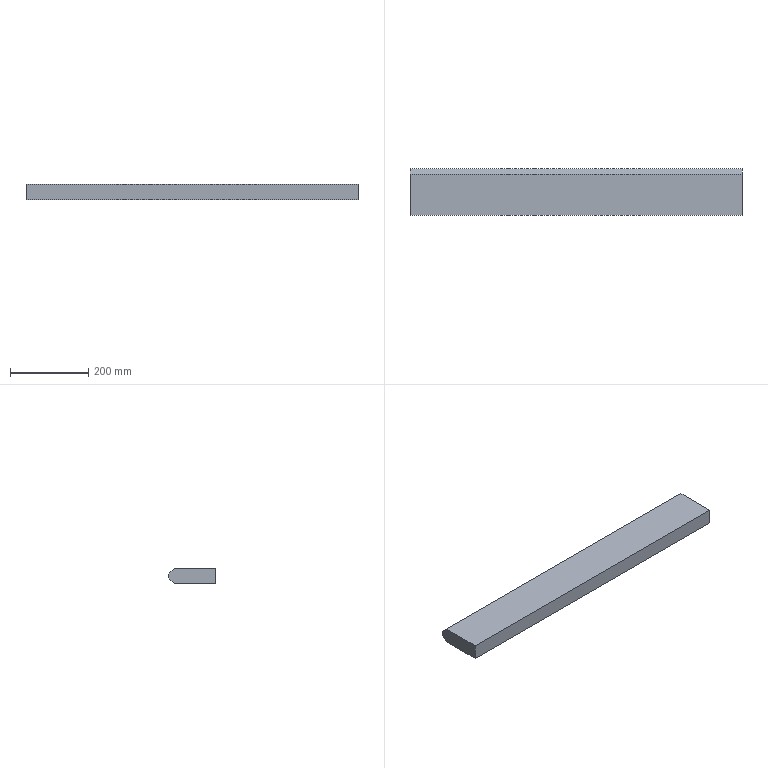Part | SolidWorks | features Chamfer 1, Extrusion 1 | 1 solid | 8 faces | box 850 x 120 x 40 mm | volume 3888750 mm3 | plane 8
STEP:
#1=CARTESIAN_POINT('',(-425.,60.,5.));
#2=VERTEX_POINT('',#1);
#3=CARTESIAN_POINT('',(-425.,60.,-5.));
#4=VERTEX_POINT('',#3);
#5=CARTESIAN_POINT('',(-425.,60.,20.));
#6=DIRECTION('',(0.,0.,-1.));
#7=VECTOR('',#6,1000.);
#8=LINE('',#5,#7);
#9=EDGE_CURVE('',#2,#4,#8,.T.);
#10=ORIENTED_EDGE('',*,*,#9,.T.);
#11=CARTESIAN_POINT('',(-425.,45.,-20.));
#12=VERTEX_POINT('',#11);
#13=CARTESIAN_POINT('',(-425.,60.,-5.));
#14=DIRECTION('',(0.,-0.7071,-0.7071));
#15=VECTOR('',#14,1000.);
#16=LINE('',#13,#15);
#17=EDGE_CURVE('',#4,#12,#16,.T.);
#18=ORIENTED_EDGE('',*,*,#17,.T.);
#19=CARTESIAN_POINT('',(-425.,-60.,-20.));
#20=VERTEX_POINT('',#19);
#21=CARTESIAN_POINT('',(-425.,-60.,-20.));
#22=DIRECTION('',(0.,-1.,0.));
#23=VECTOR('',#22,1000.);
#24=LINE('',#21,#23);
#25=EDGE_CURVE('',#12,#20,#24,.T.);
#26=ORIENTED_EDGE('',*,*,#25,.T.);
#27=CARTESIAN_POINT('',(-425.,-60.,20.));
#28=VERTEX_POINT('',#27);
#29=CARTESIAN_POINT('',(-425.,-60.,20.));
#30=DIRECTION('',(0.,0.,-1.));
#31=VECTOR('',#30,1000.);
#32=LINE('',#29,#31);
#33=EDGE_CURVE('',#28,#20,#32,.T.);
#34=ORIENTED_EDGE('',*,*,#33,.F.);
#35=CARTESIAN_POINT('',(-425.,45.,20.));
#36=VERTEX_POINT('',#35);
#37=CARTESIAN_POINT('',(-425.,-60.,20.));
#38=DIRECTION('',(0.,-1.,0.));
#39=VECTOR('',#38,1000.);
#40=LINE('',#37,#39);
#41=EDGE_CURVE('',#36,#28,#40,.T.);
#42=ORIENTED_EDGE('',*,*,#41,.F.);
#43=CARTESIAN_POINT('',(-425.,45.,20.));
#44=DIRECTION('',(0.,0.7071,-0.7071));
#45=VECTOR('',#44,1000.);
#46=LINE('',#43,#45);
#47=EDGE_CURVE('',#36,#2,#46,.T.);
#48=ORIENTED_EDGE('',*,*,#47,.T.);
#49=EDGE_LOOP('',(#10,#18,#26,#34,#42,#48));
#50=FACE_OUTER_BOUND('',#49,.T.);
#51=CARTESIAN_POINT('',(-425.,-60.,20.));
#52=DIRECTION('',(1.,0.,0.));
#53=DIRECTION('',(0.,0.,-1.));
#54=AXIS2_PLACEMENT_3D('',#51,#52,#53);
#55=PLANE('',#54);
#56=ADVANCED_FACE('',(#50),#55,.F.);
#57=CARTESIAN_POINT('',(425.,-60.,-20.));
#58=VERTEX_POINT('',#57);
#59=CARTESIAN_POINT('',(425.,-60.,-20.));
#60=DIRECTION('',(1.,0.,0.));
#61=VECTOR('',#60,1000.);
#62=LINE('',#59,#61);
#63=EDGE_CURVE('',#20,#58,#62,.T.);
#64=ORIENTED_EDGE('',*,*,#63,.T.);
#65=CARTESIAN_POINT('',(425.,-60.,20.));
#66=VERTEX_POINT('',#65);
#67=CARTESIAN_POINT('',(425.,-60.,20.));
#68=DIRECTION('',(0.,0.,-1.));
#69=VECTOR('',#68,1000.);
#70=LINE('',#67,#69);
#71=EDGE_CURVE('',#66,#58,#70,.T.);
#72=ORIENTED_EDGE('',*,*,#71,.F.);
#73=CARTESIAN_POINT('',(425.,-60.,20.));
#74=DIRECTION('',(1.,0.,0.));
#75=VECTOR('',#74,1000.);
#76=LINE('',#73,#75);
#77=EDGE_CURVE('',#28,#66,#76,.T.);
#78=ORIENTED_EDGE('',*,*,#77,.F.);
#79=ORIENTED_EDGE('',*,*,#33,.T.);
#80=EDGE_LOOP('',(#64,#72,#78,#79));
#81=FACE_OUTER_BOUND('',#80,.T.);
#82=CARTESIAN_POINT('',(425.,-60.,20.));
#83=DIRECTION('',(0.,1.,0.));
#84=DIRECTION('',(-1.,0.,0.));
#85=AXIS2_PLACEMENT_3D('',#82,#83,#84);
#86=PLANE('',#85);
#87=ADVANCED_FACE('',(#81),#86,.F.);
#88=CARTESIAN_POINT('',(425.,45.,-20.));
#89=VERTEX_POINT('',#88);
#90=CARTESIAN_POINT('',(425.,-60.,-20.));
#91=DIRECTION('',(0.,1.,0.));
#92=VECTOR('',#91,1000.);
#93=LINE('',#90,#92);
#94=EDGE_CURVE('',#58,#89,#93,.T.);
#95=ORIENTED_EDGE('',*,*,#94,.T.);
#96=CARTESIAN_POINT('',(425.,60.,-5.));
#97=VERTEX_POINT('',#96);
#98=CARTESIAN_POINT('',(425.,60.,-5.));
#99=DIRECTION('',(0.,0.7071,0.7071));
#100=VECTOR('',#99,1000.);
#101=LINE('',#98,#100);
#102=EDGE_CURVE('',#89,#97,#101,.T.);
#103=ORIENTED_EDGE('',*,*,#102,.T.);
#104=CARTESIAN_POINT('',(425.,60.,5.));
#105=VERTEX_POINT('',#104);
#106=CARTESIAN_POINT('',(425.,60.,20.));
#107=DIRECTION('',(0.,0.,-1.));
#108=VECTOR('',#107,1000.);
#109=LINE('',#106,#108);
#110=EDGE_CURVE('',#105,#97,#109,.T.);
#111=ORIENTED_EDGE('',*,*,#110,.F.);
#112=CARTESIAN_POINT('',(425.,45.,20.));
#113=VERTEX_POINT('',#112);
#114=CARTESIAN_POINT('',(425.,45.,20.));
#115=DIRECTION('',(0.,-0.7071,0.7071));
#116=VECTOR('',#115,1000.);
#117=LINE('',#114,#116);
#118=EDGE_CURVE('',#105,#113,#117,.T.);
#119=ORIENTED_EDGE('',*,*,#118,.T.);
#120=CARTESIAN_POINT('',(425.,-60.,20.));
#121=DIRECTION('',(0.,1.,0.));
#122=VECTOR('',#121,1000.);
#123=LINE('',#120,#122);
#124=EDGE_CURVE('',#66,#113,#123,.T.);
#125=ORIENTED_EDGE('',*,*,#124,.F.);
#126=ORIENTED_EDGE('',*,*,#71,.T.);
#127=EDGE_LOOP('',(#95,#103,#111,#119,#125,#126));
#128=FACE_OUTER_BOUND('',#127,.T.);
#129=CARTESIAN_POINT('',(425.,-60.,20.));
#130=DIRECTION('',(-1.,0.,0.));
#131=DIRECTION('',(0.,0.,1.));
#132=AXIS2_PLACEMENT_3D('',#129,#130,#131);
#133=PLANE('',#132);
#134=ADVANCED_FACE('',(#128),#133,.F.);
#135=ORIENTED_EDGE('',*,*,#110,.T.);
#136=CARTESIAN_POINT('',(425.,60.,-5.));
#137=DIRECTION('',(-1.,0.,0.));
#138=VECTOR('',#137,1000.);
#139=LINE('',#136,#138);
#140=EDGE_CURVE('',#97,#4,#139,.T.);
#141=ORIENTED_EDGE('',*,*,#140,.T.);
#142=ORIENTED_EDGE('',*,*,#9,.F.);
#143=CARTESIAN_POINT('',(425.,60.,5.));
#144=DIRECTION('',(1.,0.,0.));
#145=VECTOR('',#144,1000.);
#146=LINE('',#143,#145);
#147=EDGE_CURVE('',#2,#105,#146,.T.);
#148=ORIENTED_EDGE('',*,*,#147,.T.);
#149=EDGE_LOOP('',(#135,#141,#142,#148));
#150=FACE_OUTER_BOUND('',#149,.T.);
#151=CARTESIAN_POINT('',(425.,60.,20.));
#152=DIRECTION('',(0.,-1.,0.));
#153=DIRECTION('',(1.,0.,0.));
#154=AXIS2_PLACEMENT_3D('',#151,#152,#153);
#155=PLANE('',#154);
#156=ADVANCED_FACE('',(#150),#155,.F.);
#157=ORIENTED_EDGE('',*,*,#124,.T.);
#158=CARTESIAN_POINT('',(-425.,45.,20.));
#159=DIRECTION('',(-1.,0.,0.));
#160=VECTOR('',#159,1000.);
#161=LINE('',#158,#160);
#162=EDGE_CURVE('',#113,#36,#161,.T.);
#163=ORIENTED_EDGE('',*,*,#162,.T.);
#164=ORIENTED_EDGE('',*,*,#41,.T.);
#165=ORIENTED_EDGE('',*,*,#77,.T.);
#166=EDGE_LOOP('',(#157,#163,#164,#165));
#167=FACE_OUTER_BOUND('',#166,.T.);
#168=CARTESIAN_POINT('',(0.,0.,20.));
#169=DIRECTION('',(0.,0.,1.));
#170=DIRECTION('',(1.,0.,0.));
#171=AXIS2_PLACEMENT_3D('',#168,#169,#170);
#172=PLANE('',#171);
#173=ADVANCED_FACE('',(#167),#172,.T.);
#174=ORIENTED_EDGE('',*,*,#25,.F.);
#175=CARTESIAN_POINT('',(0.,45.,-20.));
#176=DIRECTION('',(1.,0.,0.));
#177=VECTOR('',#176,1000.);
#178=LINE('',#175,#177);
#179=EDGE_CURVE('',#12,#89,#178,.T.);
#180=ORIENTED_EDGE('',*,*,#179,.T.);
#181=ORIENTED_EDGE('',*,*,#94,.F.);
#182=ORIENTED_EDGE('',*,*,#63,.F.);
#183=EDGE_LOOP('',(#174,#180,#181,#182));
#184=FACE_OUTER_BOUND('',#183,.T.);
#185=CARTESIAN_POINT('',(0.,0.,-20.));
#186=DIRECTION('',(0.,0.,1.));
#187=DIRECTION('',(1.,0.,0.));
#188=AXIS2_PLACEMENT_3D('',#185,#186,#187);
#189=PLANE('',#188);
#190=ADVANCED_FACE('',(#184),#189,.F.);
#191=ORIENTED_EDGE('',*,*,#102,.F.);
#192=ORIENTED_EDGE('',*,*,#179,.F.);
#193=ORIENTED_EDGE('',*,*,#17,.F.);
#194=ORIENTED_EDGE('',*,*,#140,.F.);
#195=EDGE_LOOP('',(#191,#192,#193,#194));
#196=FACE_OUTER_BOUND('',#195,.T.);
#197=CARTESIAN_POINT('',(425.,60.,-5.));
#198=DIRECTION('',(0.,-0.7071,0.7071));
#199=DIRECTION('',(-1.,0.,0.));
#200=AXIS2_PLACEMENT_3D('',#197,#198,#199);
#201=PLANE('',#200);
#202=ADVANCED_FACE('',(#196),#201,.F.);
#203=ORIENTED_EDGE('',*,*,#118,.F.);
#204=ORIENTED_EDGE('',*,*,#147,.F.);
#205=ORIENTED_EDGE('',*,*,#47,.F.);
#206=ORIENTED_EDGE('',*,*,#162,.F.);
#207=EDGE_LOOP('',(#203,#204,#205,#206));
#208=FACE_OUTER_BOUND('',#207,.T.);
#209=CARTESIAN_POINT('',(0.,45.,20.));
#210=DIRECTION('',(0.,0.7071,0.7071));
#211=DIRECTION('',(1.,0.,0.));
#212=AXIS2_PLACEMENT_3D('',#209,#210,#211);
#213=PLANE('',#212);
#214=ADVANCED_FACE('',(#208),#213,.T.);
#215=CLOSED_SHELL('',(#56,#87,#134,#156,#173,#190,#202,#214));
#216=MANIFOLD_SOLID_BREP('',#215);
#217=CARTESIAN_POINT('',(0.,0.,0.));
#218=DIRECTION('',(0.,0.,1.));
#219=DIRECTION('',(1.,0.,0.));
#220=AXIS2_PLACEMENT_3D('',#217,#218,#219);
#221=(LENGTH_UNIT()NAMED_UNIT(*)SI_UNIT(.MILLI.,.METRE.));
#222=UNCERTAINTY_MEASURE_WITH_UNIT(LENGTH_MEASURE(0.00001),#221,'','');
#223=(NAMED_UNIT(*)PLANE_ANGLE_UNIT()SI_UNIT($,.RADIAN.));
#224=(NAMED_UNIT(*)SI_UNIT($,.STERADIAN.)SOLID_ANGLE_UNIT());
#225=(GEOMETRIC_REPRESENTATION_CONTEXT(3)GLOBAL_UNCERTAINTY_ASSIGNED_CONTEXT((#222))GLOBAL_UNIT_ASSIGNED_CONTEXT((#221,#223,#224))REPRESENTATION_CONTEXT('',''));
#226=ADVANCED_BREP_SHAPE_REPRESENTATION('',(#216,#220),#225);